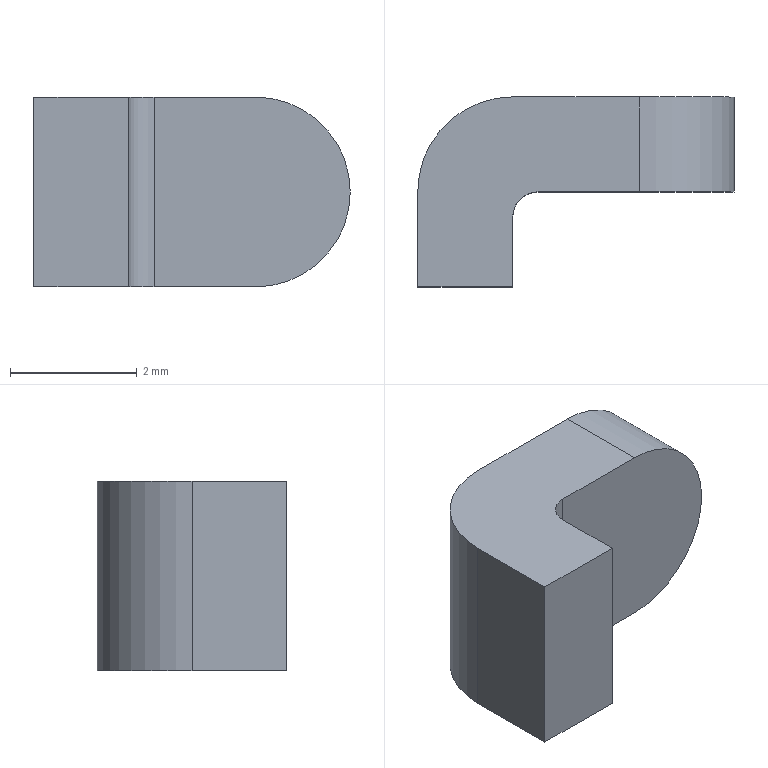Part | STEP file | LRS-150-12_X2_5F00517375-151319 | 1 solid | 10 faces | box 5 x 3 x 3 mm | volume 26.456 mm3 | plane 7 | cylinder 3 | commonest cylinder face diameters 3 x2 0.8 x1
STEP:
#1=CARTESIAN_POINT('',(0.,0.,0.));
#2=DIRECTION('',(0.,0.,1.));
#3=DIRECTION('',(1.,0.,0.));
#4=AXIS2_PLACEMENT_3D('',#1,#2,#3);
#5=CARTESIAN_POINT('',(-277.867,206.025,15.65));
#6=VERTEX_POINT('',#5);
#7=CARTESIAN_POINT('',(-276.367,206.025,17.15));
#8=VERTEX_POINT('',#7);
#9=CARTESIAN_POINT('',(-277.867,206.025,17.15));
#10=DIRECTION('',(0.,-1.,0.));
#11=DIRECTION('',(0.,0.,-1.));
#12=AXIS2_PLACEMENT_3D('',#9,#10,#11);
#13=CIRCLE('',#12,1.5);
#14=CARTESIAN_POINT('',(-277.867,204.225,17.15));
#15=DIRECTION('',(0.,1.,0.));
#16=DIRECTION('',(1.,0.,0.));
#17=AXIS2_PLACEMENT_3D('',#14,#15,#16);
#18=CYLINDRICAL_SURFACE('',#17,1.5);
#19=CARTESIAN_POINT('',(1.571,1.8));
#20=DIRECTION('',(-1.,0.));
#21=VECTOR('',#20,1.);
#22=LINE('',#19,#21);
#23=(GEOMETRIC_REPRESENTATION_CONTEXT(2)PARAMETRIC_REPRESENTATION_CONTEXT()REPRESENTATION_CONTEXT('',''));
#24=DEFINITIONAL_REPRESENTATION('',(#22),#23);
#25=PCURVE('',#18,#24);
#26=CARTESIAN_POINT('',(-279.867,206.025,15.65));
#27=DIRECTION('',(0.,-1.,0.));
#28=DIRECTION('',(0.,0.,-1.));
#29=AXIS2_PLACEMENT_3D('',#26,#27,#28);
#30=PLANE('',#29);
#31=CARTESIAN_POINT('',(-1.5,2.));
#32=DIRECTION('',(1.,0.));
#33=AXIS2_PLACEMENT_2D('',#31,#32);
#34=CIRCLE('',#33,1.5);
#35=(GEOMETRIC_REPRESENTATION_CONTEXT(2)PARAMETRIC_REPRESENTATION_CONTEXT()REPRESENTATION_CONTEXT('',''));
#36=DEFINITIONAL_REPRESENTATION('',(#34),#35);
#37=PCURVE('',#30,#36);
#38=SURFACE_CURVE('',#13,(#25,#37),.PCURVE_S1.);
#39=EDGE_CURVE('',#6,#8,#38,.T.);
#40=ORIENTED_EDGE('',*,*,#39,.F.);
#41=CARTESIAN_POINT('',(-277.867,207.525,15.65));
#42=VERTEX_POINT('',#41);
#43=CARTESIAN_POINT('',(-277.867,206.025,15.65));
#44=DIRECTION('',(0.,1.,0.));
#45=VECTOR('',#44,1.);
#46=LINE('',#43,#45);
#47=CARTESIAN_POINT('',(1.571,1.8));
#48=DIRECTION('',(0.,1.));
#49=VECTOR('',#48,1.);
#50=LINE('',#47,#49);
#51=(GEOMETRIC_REPRESENTATION_CONTEXT(2)PARAMETRIC_REPRESENTATION_CONTEXT()REPRESENTATION_CONTEXT('',''));
#52=DEFINITIONAL_REPRESENTATION('',(#50),#51);
#53=PCURVE('',#18,#52);
#54=CARTESIAN_POINT('',(-281.367,204.525,15.65));
#55=DIRECTION('',(0.,0.,-1.));
#56=DIRECTION('',(-1.,0.,0.));
#57=AXIS2_PLACEMENT_3D('',#54,#55,#56);
#58=PLANE('',#57);
#59=CARTESIAN_POINT('',(-3.5,1.5));
#60=DIRECTION('',(0.,1.));
#61=VECTOR('',#60,1.);
#62=LINE('',#59,#61);
#63=(GEOMETRIC_REPRESENTATION_CONTEXT(2)PARAMETRIC_REPRESENTATION_CONTEXT()REPRESENTATION_CONTEXT('',''));
#64=DEFINITIONAL_REPRESENTATION('',(#62),#63);
#65=PCURVE('',#58,#64);
#66=SURFACE_CURVE('',#46,(#53,#65),.PCURVE_S1.);
#67=EDGE_CURVE('',#6,#42,#66,.T.);
#68=ORIENTED_EDGE('',*,*,#67,.T.);
#69=CARTESIAN_POINT('',(-276.367,207.525,17.15));
#70=VERTEX_POINT('',#69);
#71=CARTESIAN_POINT('',(-277.867,207.525,17.15));
#72=DIRECTION('',(0.,1.,0.));
#73=DIRECTION('',(1.,0.,0.));
#74=AXIS2_PLACEMENT_3D('',#71,#72,#73);
#75=CIRCLE('',#74,1.5);
#76=CARTESIAN_POINT('',(0.,3.3));
#77=DIRECTION('',(1.,0.));
#78=VECTOR('',#77,1.);
#79=LINE('',#76,#78);
#80=(GEOMETRIC_REPRESENTATION_CONTEXT(2)PARAMETRIC_REPRESENTATION_CONTEXT()REPRESENTATION_CONTEXT('',''));
#81=DEFINITIONAL_REPRESENTATION('',(#79),#80);
#82=PCURVE('',#18,#81);
#83=CARTESIAN_POINT('',(-282.729,207.525,17.452));
#84=DIRECTION('',(0.,1.,0.));
#85=DIRECTION('',(1.,0.,0.));
#86=AXIS2_PLACEMENT_3D('',#83,#84,#85);
#87=PLANE('',#86);
#88=CARTESIAN_POINT('',(4.862,0.302));
#89=DIRECTION('',(1.,0.));
#90=AXIS2_PLACEMENT_2D('',#88,#89);
#91=CIRCLE('',#90,1.5);
#92=(GEOMETRIC_REPRESENTATION_CONTEXT(2)PARAMETRIC_REPRESENTATION_CONTEXT()REPRESENTATION_CONTEXT('',''));
#93=DEFINITIONAL_REPRESENTATION('',(#91),#92);
#94=PCURVE('',#87,#93);
#95=SURFACE_CURVE('',#75,(#82,#94),.PCURVE_S1.);
#96=EDGE_CURVE('',#70,#42,#95,.T.);
#97=ORIENTED_EDGE('',*,*,#96,.F.);
#98=CARTESIAN_POINT('',(-277.867,207.525,18.65));
#99=VERTEX_POINT('',#98);
#100=CARTESIAN_POINT('',(-277.867,207.525,17.15));
#101=DIRECTION('',(0.,1.,0.));
#102=DIRECTION('',(0.,0.,1.));
#103=AXIS2_PLACEMENT_3D('',#100,#101,#102);
#104=CIRCLE('',#103,1.5);
#105=CARTESIAN_POINT('',(-1.571,3.3));
#106=DIRECTION('',(1.,0.));
#107=VECTOR('',#106,1.);
#108=LINE('',#105,#107);
#109=(GEOMETRIC_REPRESENTATION_CONTEXT(2)PARAMETRIC_REPRESENTATION_CONTEXT()REPRESENTATION_CONTEXT('',''));
#110=DEFINITIONAL_REPRESENTATION('',(#108),#109);
#111=PCURVE('',#18,#110);
#112=CARTESIAN_POINT('',(4.862,0.302));
#113=DIRECTION('',(0.,-1.));
#114=AXIS2_PLACEMENT_2D('',#112,#113);
#115=CIRCLE('',#114,1.5);
#116=(GEOMETRIC_REPRESENTATION_CONTEXT(2)PARAMETRIC_REPRESENTATION_CONTEXT()REPRESENTATION_CONTEXT('',''));
#117=DEFINITIONAL_REPRESENTATION('',(#115),#116);
#118=PCURVE('',#87,#117);
#119=SURFACE_CURVE('',#104,(#111,#118),.PCURVE_S1.);
#120=EDGE_CURVE('',#99,#70,#119,.T.);
#121=ORIENTED_EDGE('',*,*,#120,.F.);
#122=CARTESIAN_POINT('',(-277.867,206.025,18.65));
#123=VERTEX_POINT('',#122);
#124=CARTESIAN_POINT('',(-277.867,207.525,18.65));
#125=DIRECTION('',(0.,-1.,0.));
#126=VECTOR('',#125,1.);
#127=LINE('',#124,#126);
#128=CARTESIAN_POINT('',(-1.571,3.3));
#129=DIRECTION('',(0.,-1.));
#130=VECTOR('',#129,1.);
#131=LINE('',#128,#130);
#132=(GEOMETRIC_REPRESENTATION_CONTEXT(2)PARAMETRIC_REPRESENTATION_CONTEXT()REPRESENTATION_CONTEXT('',''));
#133=DEFINITIONAL_REPRESENTATION('',(#131),#132);
#134=PCURVE('',#18,#133);
#135=CARTESIAN_POINT('',(-279.867,204.525,18.65));
#136=DIRECTION('',(0.,0.,1.));
#137=DIRECTION('',(1.,0.,0.));
#138=AXIS2_PLACEMENT_3D('',#135,#136,#137);
#139=PLANE('',#138);
#140=CARTESIAN_POINT('',(2.,3.));
#141=DIRECTION('',(0.,-1.));
#142=VECTOR('',#141,1.);
#143=LINE('',#140,#142);
#144=(GEOMETRIC_REPRESENTATION_CONTEXT(2)PARAMETRIC_REPRESENTATION_CONTEXT()REPRESENTATION_CONTEXT('',''));
#145=DEFINITIONAL_REPRESENTATION('',(#143),#144);
#146=PCURVE('',#139,#145);
#147=SURFACE_CURVE('',#127,(#134,#146),.PCURVE_S1.);
#148=EDGE_CURVE('',#99,#123,#147,.T.);
#149=ORIENTED_EDGE('',*,*,#148,.T.);
#150=CARTESIAN_POINT('',(-277.867,206.025,17.15));
#151=DIRECTION('',(0.,-1.,0.));
#152=DIRECTION('',(1.,0.,0.));
#153=AXIS2_PLACEMENT_3D('',#150,#151,#152);
#154=CIRCLE('',#153,1.5);
#155=CARTESIAN_POINT('',(0.,1.8));
#156=DIRECTION('',(-1.,0.));
#157=VECTOR('',#156,1.);
#158=LINE('',#155,#157);
#159=(GEOMETRIC_REPRESENTATION_CONTEXT(2)PARAMETRIC_REPRESENTATION_CONTEXT()REPRESENTATION_CONTEXT('',''));
#160=DEFINITIONAL_REPRESENTATION('',(#158),#159);
#161=PCURVE('',#18,#160);
#162=CARTESIAN_POINT('',(-1.5,2.));
#163=DIRECTION('',(0.,1.));
#164=AXIS2_PLACEMENT_2D('',#162,#163);
#165=CIRCLE('',#164,1.5);
#166=(GEOMETRIC_REPRESENTATION_CONTEXT(2)PARAMETRIC_REPRESENTATION_CONTEXT()REPRESENTATION_CONTEXT('',''));
#167=DEFINITIONAL_REPRESENTATION('',(#165),#166);
#168=PCURVE('',#30,#167);
#169=SURFACE_CURVE('',#154,(#161,#168),.PCURVE_S1.);
#170=EDGE_CURVE('',#8,#123,#169,.T.);
#171=ORIENTED_EDGE('',*,*,#170,.F.);
#172=EDGE_LOOP('',(#40,#68,#97,#121,#149,#171));
#173=FACE_BOUND('',#172,.T.);
#174=ADVANCED_FACE('',(#173),#18,.T.);
#175=CARTESIAN_POINT('',(-279.467,206.025,15.65));
#176=VERTEX_POINT('',#175);
#177=CARTESIAN_POINT('',(-279.467,206.025,15.65));
#178=DIRECTION('',(1.,0.,0.));
#179=VECTOR('',#178,1.);
#180=LINE('',#177,#179);
#181=CARTESIAN_POINT('',(0.,0.4));
#182=DIRECTION('',(0.,1.));
#183=VECTOR('',#182,1.);
#184=LINE('',#181,#183);
#185=(GEOMETRIC_REPRESENTATION_CONTEXT(2)PARAMETRIC_REPRESENTATION_CONTEXT()REPRESENTATION_CONTEXT('',''));
#186=DEFINITIONAL_REPRESENTATION('',(#184),#185);
#187=PCURVE('',#30,#186);
#188=CARTESIAN_POINT('',(-1.9,1.5));
#189=DIRECTION('',(-1.,0.));
#190=VECTOR('',#189,1.);
#191=LINE('',#188,#190);
#192=(GEOMETRIC_REPRESENTATION_CONTEXT(2)PARAMETRIC_REPRESENTATION_CONTEXT()REPRESENTATION_CONTEXT('',''));
#193=DEFINITIONAL_REPRESENTATION('',(#191),#192);
#194=PCURVE('',#58,#193);
#195=SURFACE_CURVE('',#180,(#187,#194),.PCURVE_S1.);
#196=EDGE_CURVE('',#176,#6,#195,.T.);
#197=ORIENTED_EDGE('',*,*,#196,.F.);
#198=CARTESIAN_POINT('',(-279.467,206.025,18.65));
#199=VERTEX_POINT('',#198);
#200=CARTESIAN_POINT('',(-279.467,206.025,15.65));
#201=DIRECTION('',(0.,0.,1.));
#202=VECTOR('',#201,1.);
#203=LINE('',#200,#202);
#204=CARTESIAN_POINT('',(0.,0.4));
#205=DIRECTION('',(-1.,0.));
#206=VECTOR('',#205,1.);
#207=LINE('',#204,#206);
#208=(GEOMETRIC_REPRESENTATION_CONTEXT(2)PARAMETRIC_REPRESENTATION_CONTEXT()REPRESENTATION_CONTEXT('',''));
#209=DEFINITIONAL_REPRESENTATION('',(#207),#208);
#210=PCURVE('',#30,#209);
#211=CARTESIAN_POINT('',(-279.467,205.625,17.452));
#212=DIRECTION('',(0.,0.,-1.));
#213=DIRECTION('',(-1.,0.,0.));
#214=AXIS2_PLACEMENT_3D('',#211,#212,#213);
#215=CYLINDRICAL_SURFACE('',#214,0.4);
#216=CARTESIAN_POINT('',(1.571,1.802));
#217=DIRECTION('',(0.,-1.));
#218=VECTOR('',#217,1.);
#219=LINE('',#216,#218);
#220=(GEOMETRIC_REPRESENTATION_CONTEXT(2)PARAMETRIC_REPRESENTATION_CONTEXT()REPRESENTATION_CONTEXT('',''));
#221=DEFINITIONAL_REPRESENTATION('',(#219),#220);
#222=PCURVE('',#215,#221);
#223=SURFACE_CURVE('',#203,(#210,#222),.PCURVE_S1.);
#224=EDGE_CURVE('',#176,#199,#223,.T.);
#225=ORIENTED_EDGE('',*,*,#224,.T.);
#226=CARTESIAN_POINT('',(-279.467,206.025,18.65));
#227=DIRECTION('',(1.,0.,0.));
#228=VECTOR('',#227,1.);
#229=LINE('',#226,#228);
#230=CARTESIAN_POINT('',(-3.,0.4));
#231=DIRECTION('',(0.,1.));
#232=VECTOR('',#231,1.);
#233=LINE('',#230,#232);
#234=(GEOMETRIC_REPRESENTATION_CONTEXT(2)PARAMETRIC_REPRESENTATION_CONTEXT()REPRESENTATION_CONTEXT('',''));
#235=DEFINITIONAL_REPRESENTATION('',(#233),#234);
#236=PCURVE('',#30,#235);
#237=CARTESIAN_POINT('',(0.4,1.5));
#238=DIRECTION('',(1.,0.));
#239=VECTOR('',#238,1.);
#240=LINE('',#237,#239);
#241=(GEOMETRIC_REPRESENTATION_CONTEXT(2)PARAMETRIC_REPRESENTATION_CONTEXT()REPRESENTATION_CONTEXT('',''));
#242=DEFINITIONAL_REPRESENTATION('',(#240),#241);
#243=PCURVE('',#139,#242);
#244=SURFACE_CURVE('',#229,(#236,#243),.PCURVE_S1.);
#245=EDGE_CURVE('',#199,#123,#244,.T.);
#246=ORIENTED_EDGE('',*,*,#245,.T.);
#247=ORIENTED_EDGE('',*,*,#170,.F.);
#248=ORIENTED_EDGE('',*,*,#39,.F.);
#249=EDGE_LOOP('',(#197,#225,#246,#247,#248));
#250=FACE_BOUND('',#249,.F.);
#251=ADVANCED_FACE('',(#250),#30,.T.);
#252=CARTESIAN_POINT('',(-281.367,204.525,15.65));
#253=VERTEX_POINT('',#252);
#254=CARTESIAN_POINT('',(-281.367,206.025,15.65));
#255=VERTEX_POINT('',#254);
#256=CARTESIAN_POINT('',(-281.367,204.525,15.65));
#257=DIRECTION('',(0.,1.,0.));
#258=VECTOR('',#257,1.);
#259=LINE('',#256,#258);
#260=CARTESIAN_POINT('',(0.,0.));
#261=DIRECTION('',(0.,1.));
#262=VECTOR('',#261,1.);
#263=LINE('',#260,#262);
#264=(GEOMETRIC_REPRESENTATION_CONTEXT(2)PARAMETRIC_REPRESENTATION_CONTEXT()REPRESENTATION_CONTEXT('',''));
#265=DEFINITIONAL_REPRESENTATION('',(#263),#264);
#266=PCURVE('',#58,#265);
#267=CARTESIAN_POINT('',(-281.367,204.525,18.65));
#268=DIRECTION('',(-1.,0.,0.));
#269=DIRECTION('',(0.,0.,1.));
#270=AXIS2_PLACEMENT_3D('',#267,#268,#269);
#271=PLANE('',#270);
#272=CARTESIAN_POINT('',(-3.,0.));
#273=DIRECTION('',(0.,1.));
#274=VECTOR('',#273,1.);
#275=LINE('',#272,#274);
#276=(GEOMETRIC_REPRESENTATION_CONTEXT(2)PARAMETRIC_REPRESENTATION_CONTEXT()REPRESENTATION_CONTEXT('',''));
#277=DEFINITIONAL_REPRESENTATION('',(#275),#276);
#278=PCURVE('',#271,#277);
#279=SURFACE_CURVE('',#259,(#266,#278),.PCURVE_S1.);
#280=EDGE_CURVE('',#253,#255,#279,.T.);
#281=ORIENTED_EDGE('',*,*,#280,.F.);
#282=CARTESIAN_POINT('',(-279.867,204.525,15.65));
#283=VERTEX_POINT('',#282);
#284=CARTESIAN_POINT('',(-279.867,204.525,15.65));
#285=DIRECTION('',(-1.,0.,0.));
#286=VECTOR('',#285,1.);
#287=LINE('',#284,#286);
#288=CARTESIAN_POINT('',(-1.5,0.));
#289=DIRECTION('',(1.,0.));
#290=VECTOR('',#289,1.);
#291=LINE('',#288,#290);
#292=(GEOMETRIC_REPRESENTATION_CONTEXT(2)PARAMETRIC_REPRESENTATION_CONTEXT()REPRESENTATION_CONTEXT('',''));
#293=DEFINITIONAL_REPRESENTATION('',(#291),#292);
#294=PCURVE('',#58,#293);
#295=CARTESIAN_POINT('',(-282.729,204.525,17.452));
#296=DIRECTION('',(0.,1.,0.));
#297=DIRECTION('',(1.,0.,0.));
#298=AXIS2_PLACEMENT_3D('',#295,#296,#297);
#299=PLANE('',#298);
#300=CARTESIAN_POINT('',(2.862,1.802));
#301=DIRECTION('',(-1.,0.));
#302=VECTOR('',#301,1.);
#303=LINE('',#300,#302);
#304=(GEOMETRIC_REPRESENTATION_CONTEXT(2)PARAMETRIC_REPRESENTATION_CONTEXT()REPRESENTATION_CONTEXT('',''));
#305=DEFINITIONAL_REPRESENTATION('',(#303),#304);
#306=PCURVE('',#299,#305);
#307=SURFACE_CURVE('',#287,(#294,#306),.PCURVE_S1.);
#308=EDGE_CURVE('',#283,#253,#307,.T.);
#309=ORIENTED_EDGE('',*,*,#308,.F.);
#310=CARTESIAN_POINT('',(-279.867,205.625,15.65));
#311=VERTEX_POINT('',#310);
#312=CARTESIAN_POINT('',(-279.867,204.525,15.65));
#313=DIRECTION('',(0.,1.,0.));
#314=VECTOR('',#313,1.);
#315=LINE('',#312,#314);
#316=CARTESIAN_POINT('',(-1.5,0.));
#317=DIRECTION('',(0.,1.));
#318=VECTOR('',#317,1.);
#319=LINE('',#316,#318);
#320=(GEOMETRIC_REPRESENTATION_CONTEXT(2)PARAMETRIC_REPRESENTATION_CONTEXT()REPRESENTATION_CONTEXT('',''));
#321=DEFINITIONAL_REPRESENTATION('',(#319),#320);
#322=PCURVE('',#58,#321);
#323=CARTESIAN_POINT('',(-279.867,204.525,15.65));
#324=DIRECTION('',(1.,0.,0.));
#325=DIRECTION('',(0.,0.,-1.));
#326=AXIS2_PLACEMENT_3D('',#323,#324,#325);
#327=PLANE('',#326);
#328=CARTESIAN_POINT('',(0.,0.));
#329=DIRECTION('',(0.,1.));
#330=VECTOR('',#329,1.);
#331=LINE('',#328,#330);
#332=(GEOMETRIC_REPRESENTATION_CONTEXT(2)PARAMETRIC_REPRESENTATION_CONTEXT()REPRESENTATION_CONTEXT('',''));
#333=DEFINITIONAL_REPRESENTATION('',(#331),#332);
#334=PCURVE('',#327,#333);
#335=SURFACE_CURVE('',#315,(#322,#334),.PCURVE_S1.);
#336=EDGE_CURVE('',#283,#311,#335,.T.);
#337=ORIENTED_EDGE('',*,*,#336,.T.);
#338=CARTESIAN_POINT('',(-279.467,205.625,15.65));
#339=DIRECTION('',(0.,0.,1.));
#340=DIRECTION('',(0.,1.,0.));
#341=AXIS2_PLACEMENT_3D('',#338,#339,#340);
#342=CIRCLE('',#341,0.4);
#343=CARTESIAN_POINT('',(-1.9,1.5));
#344=CARTESIAN_POINT('',(-1.207,1.5));
#345=CARTESIAN_POINT('',(-1.554,0.9));
#346=CARTESIAN_POINT('',(-1.9,0.3));
#347=CARTESIAN_POINT('',(-2.246,0.9));
#348=CARTESIAN_POINT('',(-2.593,1.5));
#349=CARTESIAN_POINT('',(-1.9,1.5));
#350=(BOUNDED_CURVE()B_SPLINE_CURVE(2,(#343,#344,#345,#346,#347,#348,#349),.UNSPECIFIED.,.T.,.F.)B_SPLINE_CURVE_WITH_KNOTS((1,2,2,2,2,1),(-2.094,0.,2.094,4.189,6.283,8.378),.UNSPECIFIED.)CURVE()GEOMETRIC_REPRESENTATION_ITEM()RATIONAL_B_SPLINE_CURVE((1.,0.5,1.,0.5,1.,0.5,1.))REPRESENTATION_ITEM(''));
#351=(GEOMETRIC_REPRESENTATION_CONTEXT(2)PARAMETRIC_REPRESENTATION_CONTEXT()REPRESENTATION_CONTEXT('',''));
#352=DEFINITIONAL_REPRESENTATION('',(#350),#351);
#353=PCURVE('',#58,#352);
#354=CARTESIAN_POINT('',(1.571,1.802));
#355=DIRECTION('',(-1.,0.));
#356=VECTOR('',#355,1.);
#357=LINE('',#354,#356);
#358=(GEOMETRIC_REPRESENTATION_CONTEXT(2)PARAMETRIC_REPRESENTATION_CONTEXT()REPRESENTATION_CONTEXT('',''));
#359=DEFINITIONAL_REPRESENTATION('',(#357),#358);
#360=PCURVE('',#215,#359);
#361=SURFACE_CURVE('',#342,(#353,#360),.PCURVE_S1.);
#362=EDGE_CURVE('',#176,#311,#361,.T.);
#363=ORIENTED_EDGE('',*,*,#362,.F.);
#364=ORIENTED_EDGE('',*,*,#196,.T.);
#365=ORIENTED_EDGE('',*,*,#67,.T.);
#366=CARTESIAN_POINT('',(-279.867,207.525,15.65));
#367=VERTEX_POINT('',#366);
#368=CARTESIAN_POINT('',(-277.867,207.525,15.65));
#369=DIRECTION('',(-1.,0.,0.));
#370=VECTOR('',#369,1.);
#371=LINE('',#368,#370);
#372=CARTESIAN_POINT('',(-3.5,3.));
#373=DIRECTION('',(1.,0.));
#374=VECTOR('',#373,1.);
#375=LINE('',#372,#374);
#376=(GEOMETRIC_REPRESENTATION_CONTEXT(2)PARAMETRIC_REPRESENTATION_CONTEXT()REPRESENTATION_CONTEXT('',''));
#377=DEFINITIONAL_REPRESENTATION('',(#375),#376);
#378=PCURVE('',#58,#377);
#379=CARTESIAN_POINT('',(4.862,1.802));
#380=DIRECTION('',(-1.,0.));
#381=VECTOR('',#380,1.);
#382=LINE('',#379,#381);
#383=(GEOMETRIC_REPRESENTATION_CONTEXT(2)PARAMETRIC_REPRESENTATION_CONTEXT()REPRESENTATION_CONTEXT('',''));
#384=DEFINITIONAL_REPRESENTATION('',(#382),#383);
#385=PCURVE('',#87,#384);
#386=SURFACE_CURVE('',#371,(#378,#385),.PCURVE_S1.);
#387=EDGE_CURVE('',#42,#367,#386,.T.);
#388=ORIENTED_EDGE('',*,*,#387,.T.);
#389=CARTESIAN_POINT('',(-279.867,206.025,15.65));
#390=DIRECTION('',(0.,0.,-1.));
#391=DIRECTION('',(-1.,0.,0.));
#392=AXIS2_PLACEMENT_3D('',#389,#390,#391);
#393=CIRCLE('',#392,1.5);
#394=CARTESIAN_POINT('',(-1.5,1.5));
#395=DIRECTION('',(1.,0.));
#396=AXIS2_PLACEMENT_2D('',#394,#395);
#397=CIRCLE('',#396,1.5);
#398=(GEOMETRIC_REPRESENTATION_CONTEXT(2)PARAMETRIC_REPRESENTATION_CONTEXT()REPRESENTATION_CONTEXT('',''));
#399=DEFINITIONAL_REPRESENTATION('',(#397),#398);
#400=PCURVE('',#58,#399);
#401=CARTESIAN_POINT('',(-279.867,206.025,17.452));
#402=DIRECTION('',(0.,0.,1.));
#403=DIRECTION('',(1.,0.,0.));
#404=AXIS2_PLACEMENT_3D('',#401,#402,#403);
#405=CYLINDRICAL_SURFACE('',#404,1.5);
#406=CARTESIAN_POINT('',(3.142,-1.802));
#407=DIRECTION('',(-1.,0.));
#408=VECTOR('',#407,1.);
#409=LINE('',#406,#408);
#410=(GEOMETRIC_REPRESENTATION_CONTEXT(2)PARAMETRIC_REPRESENTATION_CONTEXT()REPRESENTATION_CONTEXT('',''));
#411=DEFINITIONAL_REPRESENTATION('',(#409),#410);
#412=PCURVE('',#405,#411);
#413=SURFACE_CURVE('',#393,(#400,#412),.PCURVE_S1.);
#414=EDGE_CURVE('',#255,#367,#413,.T.);
#415=ORIENTED_EDGE('',*,*,#414,.F.);
#416=EDGE_LOOP('',(#281,#309,#337,#363,#364,#365,#388,#415));
#417=FACE_BOUND('',#416,.F.);
#418=ADVANCED_FACE('',(#417),#58,.T.);
#419=CARTESIAN_POINT('',(-281.367,204.525,18.65));
#420=VERTEX_POINT('',#419);
#421=CARTESIAN_POINT('',(-281.367,206.025,18.65));
#422=VERTEX_POINT('',#421);
#423=CARTESIAN_POINT('',(-281.367,204.525,18.65));
#424=DIRECTION('',(0.,1.,0.));
#425=VECTOR('',#424,1.);
#426=LINE('',#423,#425);
#427=CARTESIAN_POINT('',(0.,0.));
#428=DIRECTION('',(0.,1.));
#429=VECTOR('',#428,1.);
#430=LINE('',#427,#429);
#431=(GEOMETRIC_REPRESENTATION_CONTEXT(2)PARAMETRIC_REPRESENTATION_CONTEXT()REPRESENTATION_CONTEXT('',''));
#432=DEFINITIONAL_REPRESENTATION('',(#430),#431);
#433=PCURVE('',#271,#432);
#434=CARTESIAN_POINT('',(-1.5,0.));
#435=DIRECTION('',(0.,1.));
#436=VECTOR('',#435,1.);
#437=LINE('',#434,#436);
#438=(GEOMETRIC_REPRESENTATION_CONTEXT(2)PARAMETRIC_REPRESENTATION_CONTEXT()REPRESENTATION_CONTEXT('',''));
#439=DEFINITIONAL_REPRESENTATION('',(#437),#438);
#440=PCURVE('',#139,#439);
#441=SURFACE_CURVE('',#426,(#433,#440),.PCURVE_S1.);
#442=EDGE_CURVE('',#420,#422,#441,.T.);
#443=ORIENTED_EDGE('',*,*,#442,.F.);
#444=CARTESIAN_POINT('',(-281.367,204.525,15.65));
#445=DIRECTION('',(0.,0.,1.));
#446=VECTOR('',#445,1.);
#447=LINE('',#444,#446);
#448=CARTESIAN_POINT('',(-3.,0.));
#449=DIRECTION('',(1.,0.));
#450=VECTOR('',#449,1.);
#451=LINE('',#448,#450);
#452=(GEOMETRIC_REPRESENTATION_CONTEXT(2)PARAMETRIC_REPRESENTATION_CONTEXT()REPRESENTATION_CONTEXT('',''));
#453=DEFINITIONAL_REPRESENTATION('',(#451),#452);
#454=PCURVE('',#271,#453);
#455=CARTESIAN_POINT('',(1.362,1.802));
#456=DIRECTION('',(0.,-1.));
#457=VECTOR('',#456,1.);
#458=LINE('',#455,#457);
#459=(GEOMETRIC_REPRESENTATION_CONTEXT(2)PARAMETRIC_REPRESENTATION_CONTEXT()REPRESENTATION_CONTEXT('',''));
#460=DEFINITIONAL_REPRESENTATION('',(#458),#459);
#461=PCURVE('',#299,#460);
#462=SURFACE_CURVE('',#447,(#454,#461),.PCURVE_S1.);
#463=EDGE_CURVE('',#253,#420,#462,.T.);
#464=ORIENTED_EDGE('',*,*,#463,.F.);
#465=ORIENTED_EDGE('',*,*,#280,.T.);
#466=CARTESIAN_POINT('',(-281.367,206.025,15.65));
#467=DIRECTION('',(0.,0.,1.));
#468=VECTOR('',#467,1.);
#469=LINE('',#466,#468);
#470=CARTESIAN_POINT('',(-3.,1.5));
#471=DIRECTION('',(1.,0.));
#472=VECTOR('',#471,1.);
#473=LINE('',#470,#472);
#474=(GEOMETRIC_REPRESENTATION_CONTEXT(2)PARAMETRIC_REPRESENTATION_CONTEXT()REPRESENTATION_CONTEXT('',''));
#475=DEFINITIONAL_REPRESENTATION('',(#473),#474);
#476=PCURVE('',#271,#475);
#477=CARTESIAN_POINT('',(3.142,-1.802));
#478=DIRECTION('',(0.,1.));
#479=VECTOR('',#478,1.);
#480=LINE('',#477,#479);
#481=(GEOMETRIC_REPRESENTATION_CONTEXT(2)PARAMETRIC_REPRESENTATION_CONTEXT()REPRESENTATION_CONTEXT('',''));
#482=DEFINITIONAL_REPRESENTATION('',(#480),#481);
#483=PCURVE('',#405,#482);
#484=SURFACE_CURVE('',#469,(#476,#483),.PCURVE_S1.);
#485=EDGE_CURVE('',#255,#422,#484,.T.);
#486=ORIENTED_EDGE('',*,*,#485,.T.);
#487=EDGE_LOOP('',(#443,#464,#465,#486));
#488=FACE_BOUND('',#487,.F.);
#489=ADVANCED_FACE('',(#488),#271,.T.);
#490=CARTESIAN_POINT('',(-279.867,204.525,18.65));
#491=VERTEX_POINT('',#490);
#492=CARTESIAN_POINT('',(-279.867,205.625,18.65));
#493=VERTEX_POINT('',#492);
#494=CARTESIAN_POINT('',(-279.867,204.525,18.65));
#495=DIRECTION('',(0.,1.,0.));
#496=VECTOR('',#495,1.);
#497=LINE('',#494,#496);
#498=CARTESIAN_POINT('',(0.,0.));
#499=DIRECTION('',(0.,1.));
#500=VECTOR('',#499,1.);
#501=LINE('',#498,#500);
#502=(GEOMETRIC_REPRESENTATION_CONTEXT(2)PARAMETRIC_REPRESENTATION_CONTEXT()REPRESENTATION_CONTEXT('',''));
#503=DEFINITIONAL_REPRESENTATION('',(#501),#502);
#504=PCURVE('',#139,#503);
#505=CARTESIAN_POINT('',(-3.,0.));
#506=DIRECTION('',(0.,1.));
#507=VECTOR('',#506,1.);
#508=LINE('',#505,#507);
#509=(GEOMETRIC_REPRESENTATION_CONTEXT(2)PARAMETRIC_REPRESENTATION_CONTEXT()REPRESENTATION_CONTEXT('',''));
#510=DEFINITIONAL_REPRESENTATION('',(#508),#509);
#511=PCURVE('',#327,#510);
#512=SURFACE_CURVE('',#497,(#504,#511),.PCURVE_S1.);
#513=EDGE_CURVE('',#491,#493,#512,.T.);
#514=ORIENTED_EDGE('',*,*,#513,.F.);
#515=CARTESIAN_POINT('',(-281.367,204.525,18.65));
#516=DIRECTION('',(1.,0.,0.));
#517=VECTOR('',#516,1.);
#518=LINE('',#515,#517);
#519=CARTESIAN_POINT('',(-1.5,0.));
#520=DIRECTION('',(1.,0.));
#521=VECTOR('',#520,1.);
#522=LINE('',#519,#521);
#523=(GEOMETRIC_REPRESENTATION_CONTEXT(2)PARAMETRIC_REPRESENTATION_CONTEXT()REPRESENTATION_CONTEXT('',''));
#524=DEFINITIONAL_REPRESENTATION('',(#522),#523);
#525=PCURVE('',#139,#524);
#526=CARTESIAN_POINT('',(1.362,-1.198));
#527=DIRECTION('',(1.,0.));
#528=VECTOR('',#527,1.);
#529=LINE('',#526,#528);
#530=(GEOMETRIC_REPRESENTATION_CONTEXT(2)PARAMETRIC_REPRESENTATION_CONTEXT()REPRESENTATION_CONTEXT('',''));
#531=DEFINITIONAL_REPRESENTATION('',(#529),#530);
#532=PCURVE('',#299,#531);
#533=SURFACE_CURVE('',#518,(#525,#532),.PCURVE_S1.);
#534=EDGE_CURVE('',#420,#491,#533,.T.);
#535=ORIENTED_EDGE('',*,*,#534,.F.);
#536=ORIENTED_EDGE('',*,*,#442,.T.);
#537=CARTESIAN_POINT('',(-279.867,207.525,18.65));
#538=VERTEX_POINT('',#537);
#539=CARTESIAN_POINT('',(-279.867,206.025,18.65));
#540=DIRECTION('',(0.,0.,1.));
#541=DIRECTION('',(0.,1.,0.));
#542=AXIS2_PLACEMENT_3D('',#539,#540,#541);
#543=CIRCLE('',#542,1.5);
#544=CARTESIAN_POINT('',(0.,1.5));
#545=DIRECTION('',(0.,1.));
#546=AXIS2_PLACEMENT_2D('',#544,#545);
#547=CIRCLE('',#546,1.5);
#548=(GEOMETRIC_REPRESENTATION_CONTEXT(2)PARAMETRIC_REPRESENTATION_CONTEXT()REPRESENTATION_CONTEXT('',''));
#549=DEFINITIONAL_REPRESENTATION('',(#547),#548);
#550=PCURVE('',#139,#549);
#551=CARTESIAN_POINT('',(1.571,1.198));
#552=DIRECTION('',(1.,0.));
#553=VECTOR('',#552,1.);
#554=LINE('',#551,#553);
#555=(GEOMETRIC_REPRESENTATION_CONTEXT(2)PARAMETRIC_REPRESENTATION_CONTEXT()REPRESENTATION_CONTEXT('',''));
#556=DEFINITIONAL_REPRESENTATION('',(#554),#555);
#557=PCURVE('',#405,#556);
#558=SURFACE_CURVE('',#543,(#550,#557),.PCURVE_S1.);
#559=EDGE_CURVE('',#538,#422,#558,.T.);
#560=ORIENTED_EDGE('',*,*,#559,.F.);
#561=CARTESIAN_POINT('',(-279.867,207.525,18.65));
#562=DIRECTION('',(1.,0.,0.));
#563=VECTOR('',#562,1.);
#564=LINE('',#561,#563);
#565=CARTESIAN_POINT('',(0.,3.));
#566=DIRECTION('',(1.,0.));
#567=VECTOR('',#566,1.);
#568=LINE('',#565,#567);
#569=(GEOMETRIC_REPRESENTATION_CONTEXT(2)PARAMETRIC_REPRESENTATION_CONTEXT()REPRESENTATION_CONTEXT('',''));
#570=DEFINITIONAL_REPRESENTATION('',(#568),#569);
#571=PCURVE('',#139,#570);
#572=CARTESIAN_POINT('',(2.862,-1.198));
#573=DIRECTION('',(1.,0.));
#574=VECTOR('',#573,1.);
#575=LINE('',#572,#574);
#576=(GEOMETRIC_REPRESENTATION_CONTEXT(2)PARAMETRIC_REPRESENTATION_CONTEXT()REPRESENTATION_CONTEXT('',''));
#577=DEFINITIONAL_REPRESENTATION('',(#575),#576);
#578=PCURVE('',#87,#577);
#579=SURFACE_CURVE('',#564,(#571,#578),.PCURVE_S1.);
#580=EDGE_CURVE('',#538,#99,#579,.T.);
#581=ORIENTED_EDGE('',*,*,#580,.T.);
#582=ORIENTED_EDGE('',*,*,#148,.T.);
#583=ORIENTED_EDGE('',*,*,#245,.F.);
#584=CARTESIAN_POINT('',(-279.467,205.625,18.65));
#585=DIRECTION('',(0.,0.,-1.));
#586=DIRECTION('',(-1.,0.,0.));
#587=AXIS2_PLACEMENT_3D('',#584,#585,#586);
#588=CIRCLE('',#587,0.4);
#589=CARTESIAN_POINT('',(0.,1.1));
#590=CARTESIAN_POINT('',(0.,1.793));
#591=CARTESIAN_POINT('',(0.6,1.446));
#592=CARTESIAN_POINT('',(1.2,1.1));
#593=CARTESIAN_POINT('',(0.6,0.7536));
#594=CARTESIAN_POINT('',(0.,0.4072));
#595=CARTESIAN_POINT('',(0.,1.1));
#596=(BOUNDED_CURVE()B_SPLINE_CURVE(2,(#589,#590,#591,#592,#593,#594,#595),.UNSPECIFIED.,.T.,.F.)B_SPLINE_CURVE_WITH_KNOTS((1,2,2,2,2,1),(-2.094,0.,2.094,4.189,6.283,8.378),.UNSPECIFIED.)CURVE()GEOMETRIC_REPRESENTATION_ITEM()RATIONAL_B_SPLINE_CURVE((1.,0.5,1.,0.5,1.,0.5,1.))REPRESENTATION_ITEM(''));
#597=(GEOMETRIC_REPRESENTATION_CONTEXT(2)PARAMETRIC_REPRESENTATION_CONTEXT()REPRESENTATION_CONTEXT('',''));
#598=DEFINITIONAL_REPRESENTATION('',(#596),#597);
#599=PCURVE('',#139,#598);
#600=CARTESIAN_POINT('',(0.,-1.198));
#601=DIRECTION('',(1.,0.));
#602=VECTOR('',#601,1.);
#603=LINE('',#600,#602);
#604=(GEOMETRIC_REPRESENTATION_CONTEXT(2)PARAMETRIC_REPRESENTATION_CONTEXT()REPRESENTATION_CONTEXT('',''));
#605=DEFINITIONAL_REPRESENTATION('',(#603),#604);
#606=PCURVE('',#215,#605);
#607=SURFACE_CURVE('',#588,(#599,#606),.PCURVE_S1.);
#608=EDGE_CURVE('',#493,#199,#607,.T.);
#609=ORIENTED_EDGE('',*,*,#608,.F.);
#610=EDGE_LOOP('',(#514,#535,#536,#560,#581,#582,#583,#609));
#611=FACE_BOUND('',#610,.F.);
#612=ADVANCED_FACE('',(#611),#139,.T.);
#613=ORIENTED_EDGE('',*,*,#513,.T.);
#614=CARTESIAN_POINT('',(-279.867,205.625,18.65));
#615=DIRECTION('',(0.,0.,-1.));
#616=VECTOR('',#615,1.);
#617=LINE('',#614,#616);
#618=CARTESIAN_POINT('',(-3.,1.1));
#619=DIRECTION('',(1.,0.));
#620=VECTOR('',#619,1.);
#621=LINE('',#618,#620);
#622=(GEOMETRIC_REPRESENTATION_CONTEXT(2)PARAMETRIC_REPRESENTATION_CONTEXT()REPRESENTATION_CONTEXT('',''));
#623=DEFINITIONAL_REPRESENTATION('',(#621),#622);
#624=PCURVE('',#327,#623);
#625=CARTESIAN_POINT('',(0.,-1.198));
#626=DIRECTION('',(0.,1.));
#627=VECTOR('',#626,1.);
#628=LINE('',#625,#627);
#629=(GEOMETRIC_REPRESENTATION_CONTEXT(2)PARAMETRIC_REPRESENTATION_CONTEXT()REPRESENTATION_CONTEXT('',''));
#630=DEFINITIONAL_REPRESENTATION('',(#628),#629);
#631=PCURVE('',#215,#630);
#632=SURFACE_CURVE('',#617,(#624,#631),.PCURVE_S1.);
#633=EDGE_CURVE('',#493,#311,#632,.T.);
#634=ORIENTED_EDGE('',*,*,#633,.T.);
#635=ORIENTED_EDGE('',*,*,#336,.F.);
#636=CARTESIAN_POINT('',(-279.867,204.525,18.65));
#637=DIRECTION('',(0.,0.,-1.));
#638=VECTOR('',#637,1.);
#639=LINE('',#636,#638);
#640=CARTESIAN_POINT('',(-3.,0.));
#641=DIRECTION('',(1.,0.));
#642=VECTOR('',#641,1.);
#643=LINE('',#640,#642);
#644=(GEOMETRIC_REPRESENTATION_CONTEXT(2)PARAMETRIC_REPRESENTATION_CONTEXT()REPRESENTATION_CONTEXT('',''));
#645=DEFINITIONAL_REPRESENTATION('',(#643),#644);
#646=PCURVE('',#327,#645);
#647=CARTESIAN_POINT('',(2.862,-1.198));
#648=DIRECTION('',(0.,1.));
#649=VECTOR('',#648,1.);
#650=LINE('',#647,#649);
#651=(GEOMETRIC_REPRESENTATION_CONTEXT(2)PARAMETRIC_REPRESENTATION_CONTEXT()REPRESENTATION_CONTEXT('',''));
#652=DEFINITIONAL_REPRESENTATION('',(#650),#651);
#653=PCURVE('',#299,#652);
#654=SURFACE_CURVE('',#639,(#646,#653),.PCURVE_S1.);
#655=EDGE_CURVE('',#491,#283,#654,.T.);
#656=ORIENTED_EDGE('',*,*,#655,.F.);
#657=EDGE_LOOP('',(#613,#634,#635,#656));
#658=FACE_BOUND('',#657,.F.);
#659=ADVANCED_FACE('',(#658),#327,.T.);
#660=ORIENTED_EDGE('',*,*,#362,.T.);
#661=ORIENTED_EDGE('',*,*,#633,.F.);
#662=ORIENTED_EDGE('',*,*,#608,.T.);
#663=ORIENTED_EDGE('',*,*,#224,.F.);
#664=EDGE_LOOP('',(#660,#661,#662,#663));
#665=FACE_BOUND('',#664,.F.);
#666=ADVANCED_FACE('',(#665),#215,.F.);
#667=ORIENTED_EDGE('',*,*,#308,.T.);
#668=ORIENTED_EDGE('',*,*,#463,.T.);
#669=ORIENTED_EDGE('',*,*,#534,.T.);
#670=ORIENTED_EDGE('',*,*,#655,.T.);
#671=EDGE_LOOP('',(#667,#668,#669,#670));
#672=FACE_BOUND('',#671,.F.);
#673=ADVANCED_FACE('',(#672),#299,.F.);
#674=ORIENTED_EDGE('',*,*,#485,.T.);
#675=ORIENTED_EDGE('',*,*,#559,.F.);
#676=CARTESIAN_POINT('',(-279.867,207.525,18.65));
#677=DIRECTION('',(0.,0.,-1.));
#678=VECTOR('',#677,1.);
#679=LINE('',#676,#678);
#680=CARTESIAN_POINT('',(1.571,1.198));
#681=DIRECTION('',(0.,-1.));
#682=VECTOR('',#681,1.);
#683=LINE('',#680,#682);
#684=(GEOMETRIC_REPRESENTATION_CONTEXT(2)PARAMETRIC_REPRESENTATION_CONTEXT()REPRESENTATION_CONTEXT('',''));
#685=DEFINITIONAL_REPRESENTATION('',(#683),#684);
#686=PCURVE('',#405,#685);
#687=CARTESIAN_POINT('',(2.862,-1.198));
#688=DIRECTION('',(0.,1.));
#689=VECTOR('',#688,1.);
#690=LINE('',#687,#689);
#691=(GEOMETRIC_REPRESENTATION_CONTEXT(2)PARAMETRIC_REPRESENTATION_CONTEXT()REPRESENTATION_CONTEXT('',''));
#692=DEFINITIONAL_REPRESENTATION('',(#690),#691);
#693=PCURVE('',#87,#692);
#694=SURFACE_CURVE('',#679,(#686,#693),.PCURVE_S1.);
#695=EDGE_CURVE('',#538,#367,#694,.T.);
#696=ORIENTED_EDGE('',*,*,#695,.T.);
#697=ORIENTED_EDGE('',*,*,#414,.F.);
#698=EDGE_LOOP('',(#674,#675,#696,#697));
#699=FACE_BOUND('',#698,.T.);
#700=ADVANCED_FACE('',(#699),#405,.T.);
#701=ORIENTED_EDGE('',*,*,#580,.F.);
#702=ORIENTED_EDGE('',*,*,#695,.T.);
#703=ORIENTED_EDGE('',*,*,#387,.F.);
#704=ORIENTED_EDGE('',*,*,#96,.F.);
#705=ORIENTED_EDGE('',*,*,#120,.F.);
#706=EDGE_LOOP('',(#701,#702,#703,#704,#705));
#707=FACE_BOUND('',#706,.F.);
#708=ADVANCED_FACE('',(#707),#87,.T.);
#709=CLOSED_SHELL('',(#174,#251,#418,#489,#612,#659,#666,#673,#700,#708));
#710=MANIFOLD_SOLID_BREP('',#709);
#711=(LENGTH_UNIT()NAMED_UNIT(*)SI_UNIT(.MILLI.,.METRE.));
#712=UNCERTAINTY_MEASURE_WITH_UNIT(LENGTH_MEASURE(0.0000001),#711,'','');
#713=(NAMED_UNIT(*)PLANE_ANGLE_UNIT()SI_UNIT($,.RADIAN.));
#714=(NAMED_UNIT(*)SI_UNIT($,.STERADIAN.)SOLID_ANGLE_UNIT());
#715=(GEOMETRIC_REPRESENTATION_CONTEXT(3)GLOBAL_UNCERTAINTY_ASSIGNED_CONTEXT((#712))GLOBAL_UNIT_ASSIGNED_CONTEXT((#711,#713,#714))REPRESENTATION_CONTEXT('',''));
#716=ADVANCED_BREP_SHAPE_REPRESENTATION('',(#4,#710),#715);